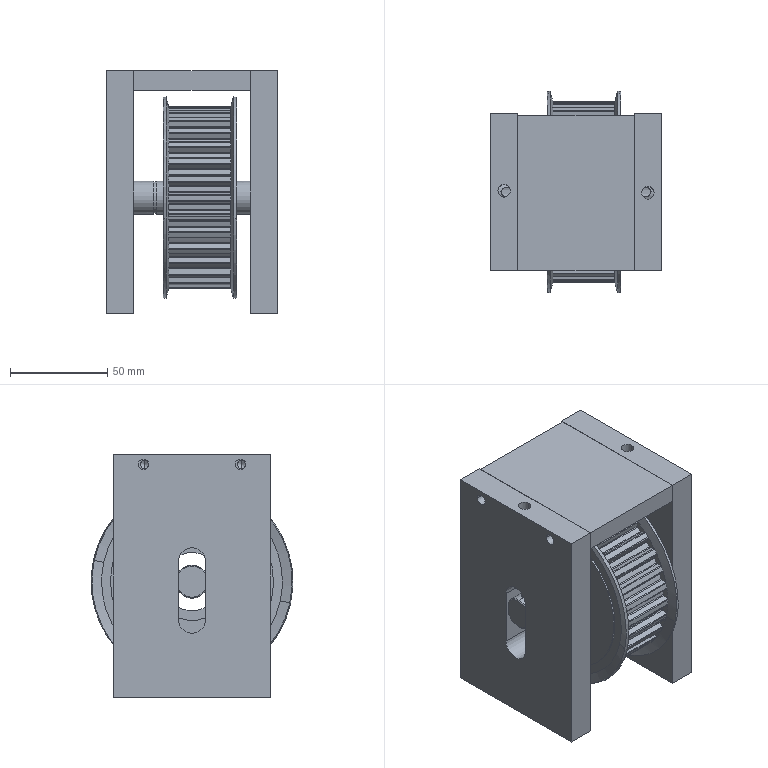Part | SolidWorks | features AEMSimFeature 1 | 5 solids | 453 faces | box 88 x 104 x 125 mm | volume 527898 mm3 | cylinder 257 | plane 162 | cone 34 | commonest cylinder face diameters 1 x70 1.2 x70 93.65 x31 87.25 x30 4.2 x8 5.5 x8